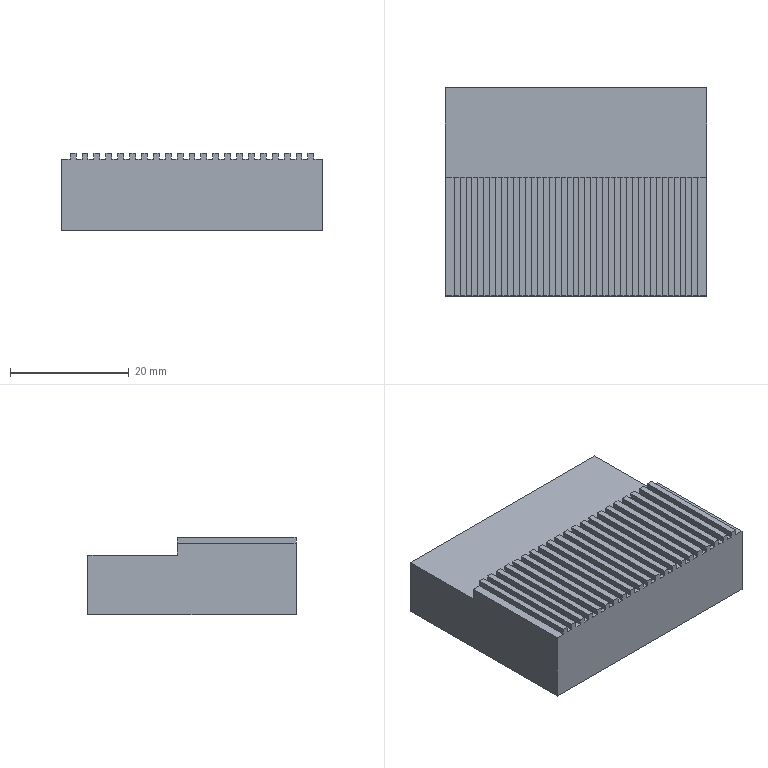Part | SolidWorks | features ICE 2, Extrusion 1, LPattern 1, MirrorPattern 1 | 1 solid | 92 faces | box 44 x 35 x 13 mm | volume 17580 mm3 | plane 92